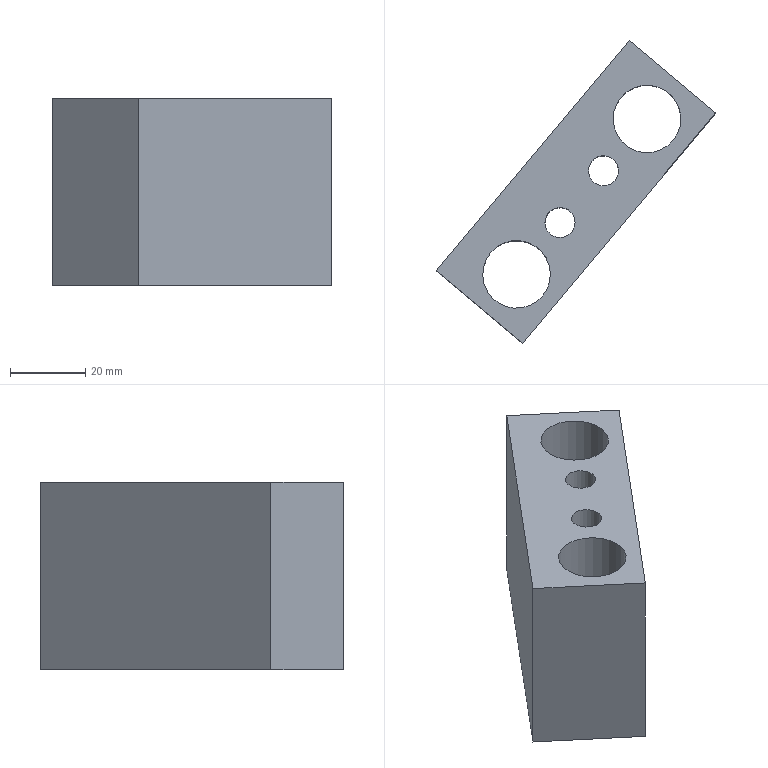Part | NX | features solid 2 | 1 solid | 10 faces | box 74.404 x 80.567 x 50 mm | volume 89527 mm3 | plane 6 | cylinder 4 | commonest cylinder face diameters 8 x2 18 x2
STEP:
#1=CARTESIAN_POINT('',(-632.193,404.46,-40.));
#2=VERTEX_POINT('',#1);
#3=CARTESIAN_POINT('',(-635.257,407.031,-40.));
#4=DIRECTION('',(0.,0.,1.));
#5=DIRECTION('',(0.766,-0.6428,0.));
#6=AXIS2_PLACEMENT_3D('',#3,#4,#5);
#7=CIRCLE('',#6,4.);
#8=EDGE_CURVE('',#2,#2,#7,.T.);
#9=ORIENTED_EDGE('',*,*,#8,.T.);
#10=EDGE_LOOP('',(#9));
#11=FACE_BOUND('',#10,.T.);
#12=CARTESIAN_POINT('',(-620.623,418.249,-40.));
#13=VERTEX_POINT('',#12);
#14=CARTESIAN_POINT('',(-623.687,420.82,-40.));
#15=DIRECTION('',(0.,0.,1.));
#16=DIRECTION('',(0.766,-0.6428,0.));
#17=AXIS2_PLACEMENT_3D('',#14,#15,#16);
#18=CIRCLE('',#17,4.);
#19=EDGE_CURVE('',#13,#13,#18,.T.);
#20=ORIENTED_EDGE('',*,*,#19,.T.);
#21=EDGE_LOOP('',(#20));
#22=FACE_BOUND('',#21,.T.);
#23=CARTESIAN_POINT('',(-605.222,428.824,-40.));
#24=VERTEX_POINT('',#23);
#25=CARTESIAN_POINT('',(-612.117,434.609,-40.));
#26=DIRECTION('',(0.,0.,1.));
#27=DIRECTION('',(0.766,-0.6428,0.));
#28=AXIS2_PLACEMENT_3D('',#25,#26,#27);
#29=CIRCLE('',#28,9.);
#30=EDGE_CURVE('',#24,#24,#29,.T.);
#31=ORIENTED_EDGE('',*,*,#30,.T.);
#32=EDGE_LOOP('',(#31));
#33=FACE_BOUND('',#32,.T.);
#34=CARTESIAN_POINT('',(-639.933,387.457,-40.));
#35=VERTEX_POINT('',#34);
#36=CARTESIAN_POINT('',(-646.827,393.242,-40.));
#37=DIRECTION('',(0.,0.,1.));
#38=DIRECTION('',(0.766,-0.6428,0.));
#39=AXIS2_PLACEMENT_3D('',#36,#37,#38);
#40=CIRCLE('',#39,9.);
#41=EDGE_CURVE('',#35,#35,#40,.T.);
#42=ORIENTED_EDGE('',*,*,#41,.T.);
#43=EDGE_LOOP('',(#42));
#44=FACE_BOUND('',#43,.T.);
#45=CARTESIAN_POINT('',(-616.783,455.495,-40.));
#46=VERTEX_POINT('',#45);
#47=CARTESIAN_POINT('',(-593.802,436.211,-40.));
#48=VERTEX_POINT('',#47);
#49=CARTESIAN_POINT('',(-569.288,415.642,-40.));
#50=DIRECTION('',(0.766,-0.6428,0.));
#51=VECTOR('',#50,1000.);
#52=LINE('',#49,#51);
#53=EDGE_CURVE('',#46,#48,#52,.T.);
#54=ORIENTED_EDGE('',*,*,#53,.T.);
#55=CARTESIAN_POINT('',(-645.225,374.927,-40.));
#56=VERTEX_POINT('',#55);
#57=CARTESIAN_POINT('',(-593.802,436.211,-40.));
#58=DIRECTION('',(-0.6428,-0.766,0.));
#59=VECTOR('',#58,1000.);
#60=LINE('',#57,#59);
#61=EDGE_CURVE('',#48,#56,#60,.T.);
#62=ORIENTED_EDGE('',*,*,#61,.T.);
#63=CARTESIAN_POINT('',(-668.206,394.211,-40.));
#64=VERTEX_POINT('',#63);
#65=CARTESIAN_POINT('',(-620.712,354.358,-40.));
#66=DIRECTION('',(0.766,-0.6428,0.));
#67=VECTOR('',#66,1000.);
#68=LINE('',#65,#67);
#69=EDGE_CURVE('',#64,#56,#68,.T.);
#70=ORIENTED_EDGE('',*,*,#69,.F.);
#71=CARTESIAN_POINT('',(-616.783,455.495,-40.));
#72=DIRECTION('',(-0.6428,-0.766,0.));
#73=VECTOR('',#72,1000.);
#74=LINE('',#71,#73);
#75=EDGE_CURVE('',#46,#64,#74,.T.);
#76=ORIENTED_EDGE('',*,*,#75,.F.);
#77=EDGE_LOOP('',(#54,#62,#70,#76));
#78=FACE_BOUND('',#77,.T.);
#79=CARTESIAN_POINT('',(-569.288,415.642,-40.));
#80=DIRECTION('',(0.,0.,-1.));
#81=DIRECTION('',(-0.6428,-0.766,0.));
#82=AXIS2_PLACEMENT_3D('',#79,#80,#81);
#83=PLANE('',#82);
#84=ADVANCED_FACE('',(#11,#22,#33,#44,#78),#83,.T.);
#85=ORIENTED_EDGE('',*,*,#69,.T.);
#86=CARTESIAN_POINT('',(-645.225,374.927,10.));
#87=VERTEX_POINT('',#86);
#88=CARTESIAN_POINT('',(-645.225,374.927,-40.));
#89=DIRECTION('',(0.,0.,1.));
#90=VECTOR('',#89,1000.);
#91=LINE('',#88,#90);
#92=EDGE_CURVE('',#56,#87,#91,.T.);
#93=ORIENTED_EDGE('',*,*,#92,.T.);
#94=CARTESIAN_POINT('',(-668.206,394.211,10.));
#95=VERTEX_POINT('',#94);
#96=CARTESIAN_POINT('',(-620.712,354.358,10.));
#97=DIRECTION('',(0.766,-0.6428,0.));
#98=VECTOR('',#97,1000.);
#99=LINE('',#96,#98);
#100=EDGE_CURVE('',#95,#87,#99,.T.);
#101=ORIENTED_EDGE('',*,*,#100,.F.);
#102=CARTESIAN_POINT('',(-668.206,394.211,-40.));
#103=DIRECTION('',(0.,0.,1.));
#104=VECTOR('',#103,1000.);
#105=LINE('',#102,#104);
#106=EDGE_CURVE('',#64,#95,#105,.T.);
#107=ORIENTED_EDGE('',*,*,#106,.F.);
#108=EDGE_LOOP('',(#85,#93,#101,#107));
#109=FACE_BOUND('',#108,.T.);
#110=CARTESIAN_POINT('',(-620.712,354.358,-40.));
#111=DIRECTION('',(-0.6428,-0.766,0.));
#112=DIRECTION('',(0.,0.,1.));
#113=AXIS2_PLACEMENT_3D('',#110,#111,#112);
#114=PLANE('',#113);
#115=ADVANCED_FACE('',(#109),#114,.T.);
#116=CARTESIAN_POINT('',(-632.193,404.46,10.));
#117=VERTEX_POINT('',#116);
#118=CARTESIAN_POINT('',(-635.257,407.031,10.));
#119=DIRECTION('',(0.,0.,1.));
#120=DIRECTION('',(0.766,-0.6428,0.));
#121=AXIS2_PLACEMENT_3D('',#118,#119,#120);
#122=CIRCLE('',#121,4.);
#123=EDGE_CURVE('',#117,#117,#122,.T.);
#124=ORIENTED_EDGE('',*,*,#123,.F.);
#125=EDGE_LOOP('',(#124));
#126=FACE_BOUND('',#125,.T.);
#127=CARTESIAN_POINT('',(-620.623,418.249,10.));
#128=VERTEX_POINT('',#127);
#129=CARTESIAN_POINT('',(-623.687,420.82,10.));
#130=DIRECTION('',(0.,0.,1.));
#131=DIRECTION('',(0.766,-0.6428,0.));
#132=AXIS2_PLACEMENT_3D('',#129,#130,#131);
#133=CIRCLE('',#132,4.);
#134=EDGE_CURVE('',#128,#128,#133,.T.);
#135=ORIENTED_EDGE('',*,*,#134,.F.);
#136=EDGE_LOOP('',(#135));
#137=FACE_BOUND('',#136,.T.);
#138=CARTESIAN_POINT('',(-605.222,428.824,10.));
#139=VERTEX_POINT('',#138);
#140=CARTESIAN_POINT('',(-612.117,434.609,10.));
#141=DIRECTION('',(0.,0.,1.));
#142=DIRECTION('',(0.766,-0.6428,0.));
#143=AXIS2_PLACEMENT_3D('',#140,#141,#142);
#144=CIRCLE('',#143,9.);
#145=EDGE_CURVE('',#139,#139,#144,.T.);
#146=ORIENTED_EDGE('',*,*,#145,.F.);
#147=EDGE_LOOP('',(#146));
#148=FACE_BOUND('',#147,.T.);
#149=CARTESIAN_POINT('',(-639.933,387.457,10.));
#150=VERTEX_POINT('',#149);
#151=CARTESIAN_POINT('',(-646.827,393.242,10.));
#152=DIRECTION('',(0.,0.,1.));
#153=DIRECTION('',(0.766,-0.6428,0.));
#154=AXIS2_PLACEMENT_3D('',#151,#152,#153);
#155=CIRCLE('',#154,9.);
#156=EDGE_CURVE('',#150,#150,#155,.T.);
#157=ORIENTED_EDGE('',*,*,#156,.F.);
#158=EDGE_LOOP('',(#157));
#159=FACE_BOUND('',#158,.T.);
#160=ORIENTED_EDGE('',*,*,#100,.T.);
#161=CARTESIAN_POINT('',(-593.802,436.211,10.));
#162=VERTEX_POINT('',#161);
#163=CARTESIAN_POINT('',(-593.802,436.211,10.));
#164=DIRECTION('',(-0.6428,-0.766,0.));
#165=VECTOR('',#164,1000.);
#166=LINE('',#163,#165);
#167=EDGE_CURVE('',#162,#87,#166,.T.);
#168=ORIENTED_EDGE('',*,*,#167,.F.);
#169=CARTESIAN_POINT('',(-616.783,455.495,10.));
#170=VERTEX_POINT('',#169);
#171=CARTESIAN_POINT('',(-569.288,415.642,10.));
#172=DIRECTION('',(0.766,-0.6428,0.));
#173=VECTOR('',#172,1000.);
#174=LINE('',#171,#173);
#175=EDGE_CURVE('',#170,#162,#174,.T.);
#176=ORIENTED_EDGE('',*,*,#175,.F.);
#177=CARTESIAN_POINT('',(-616.783,455.495,10.));
#178=DIRECTION('',(0.6428,0.766,0.));
#179=VECTOR('',#178,1000.);
#180=LINE('',#177,#179);
#181=EDGE_CURVE('',#170,#95,#180,.F.);
#182=ORIENTED_EDGE('',*,*,#181,.T.);
#183=EDGE_LOOP('',(#160,#168,#176,#182));
#184=FACE_BOUND('',#183,.T.);
#185=CARTESIAN_POINT('',(-569.288,415.642,10.));
#186=DIRECTION('',(0.,0.,-1.));
#187=DIRECTION('',(-0.6428,-0.766,0.));
#188=AXIS2_PLACEMENT_3D('',#185,#186,#187);
#189=PLANE('',#188);
#190=ADVANCED_FACE('',(#126,#137,#148,#159,#184),#189,.F.);
#191=CARTESIAN_POINT('',(-616.783,455.495,-40.));
#192=DIRECTION('',(0.,0.,-1.));
#193=VECTOR('',#192,1000.);
#194=LINE('',#191,#193);
#195=EDGE_CURVE('',#46,#170,#194,.F.);
#196=ORIENTED_EDGE('',*,*,#195,.T.);
#197=ORIENTED_EDGE('',*,*,#175,.T.);
#198=CARTESIAN_POINT('',(-593.802,436.211,-40.));
#199=DIRECTION('',(0.,0.,1.));
#200=VECTOR('',#199,1000.);
#201=LINE('',#198,#200);
#202=EDGE_CURVE('',#48,#162,#201,.T.);
#203=ORIENTED_EDGE('',*,*,#202,.F.);
#204=ORIENTED_EDGE('',*,*,#53,.F.);
#205=EDGE_LOOP('',(#196,#197,#203,#204));
#206=FACE_BOUND('',#205,.T.);
#207=CARTESIAN_POINT('',(-569.288,415.642,-40.));
#208=DIRECTION('',(-0.6428,-0.766,0.));
#209=DIRECTION('',(0.,0.,1.));
#210=AXIS2_PLACEMENT_3D('',#207,#208,#209);
#211=PLANE('',#210);
#212=ADVANCED_FACE('',(#206),#211,.F.);
#213=ORIENTED_EDGE('',*,*,#167,.T.);
#214=ORIENTED_EDGE('',*,*,#92,.F.);
#215=ORIENTED_EDGE('',*,*,#61,.F.);
#216=ORIENTED_EDGE('',*,*,#202,.T.);
#217=EDGE_LOOP('',(#213,#214,#215,#216));
#218=FACE_BOUND('',#217,.T.);
#219=CARTESIAN_POINT('',(-593.802,436.211,-40.));
#220=DIRECTION('',(0.766,-0.6428,0.));
#221=DIRECTION('',(-0.6428,-0.766,0.));
#222=AXIS2_PLACEMENT_3D('',#219,#220,#221);
#223=PLANE('',#222);
#224=ADVANCED_FACE('',(#218),#223,.T.);
#225=ORIENTED_EDGE('',*,*,#181,.F.);
#226=ORIENTED_EDGE('',*,*,#195,.F.);
#227=ORIENTED_EDGE('',*,*,#75,.T.);
#228=ORIENTED_EDGE('',*,*,#106,.T.);
#229=EDGE_LOOP('',(#225,#226,#227,#228));
#230=FACE_BOUND('',#229,.T.);
#231=CARTESIAN_POINT('',(-616.783,455.495,-40.));
#232=DIRECTION('',(0.766,-0.6428,0.));
#233=DIRECTION('',(-0.6428,-0.766,0.));
#234=AXIS2_PLACEMENT_3D('',#231,#232,#233);
#235=PLANE('',#234);
#236=ADVANCED_FACE('',(#230),#235,.F.);
#237=ORIENTED_EDGE('',*,*,#41,.F.);
#238=EDGE_LOOP('',(#237));
#239=FACE_BOUND('',#238,.T.);
#240=ORIENTED_EDGE('',*,*,#156,.T.);
#241=EDGE_LOOP('',(#240));
#242=FACE_BOUND('',#241,.T.);
#243=CARTESIAN_POINT('',(-646.827,393.242,10.));
#244=DIRECTION('',(0.,0.,-1.));
#245=DIRECTION('',(0.766,-0.6428,0.));
#246=AXIS2_PLACEMENT_3D('',#243,#244,#245);
#247=CYLINDRICAL_SURFACE('',#246,9.);
#248=ADVANCED_FACE('',(#239,#242),#247,.F.);
#249=ORIENTED_EDGE('',*,*,#30,.F.);
#250=EDGE_LOOP('',(#249));
#251=FACE_BOUND('',#250,.T.);
#252=ORIENTED_EDGE('',*,*,#145,.T.);
#253=EDGE_LOOP('',(#252));
#254=FACE_BOUND('',#253,.T.);
#255=CARTESIAN_POINT('',(-612.117,434.609,10.));
#256=DIRECTION('',(0.,0.,-1.));
#257=DIRECTION('',(0.766,-0.6428,0.));
#258=AXIS2_PLACEMENT_3D('',#255,#256,#257);
#259=CYLINDRICAL_SURFACE('',#258,9.);
#260=ADVANCED_FACE('',(#251,#254),#259,.F.);
#261=ORIENTED_EDGE('',*,*,#19,.F.);
#262=EDGE_LOOP('',(#261));
#263=FACE_BOUND('',#262,.T.);
#264=ORIENTED_EDGE('',*,*,#134,.T.);
#265=EDGE_LOOP('',(#264));
#266=FACE_BOUND('',#265,.T.);
#267=CARTESIAN_POINT('',(-623.687,420.82,10.));
#268=DIRECTION('',(0.,0.,-1.));
#269=DIRECTION('',(0.766,-0.6428,0.));
#270=AXIS2_PLACEMENT_3D('',#267,#268,#269);
#271=CYLINDRICAL_SURFACE('',#270,4.);
#272=ADVANCED_FACE('',(#263,#266),#271,.F.);
#273=ORIENTED_EDGE('',*,*,#8,.F.);
#274=EDGE_LOOP('',(#273));
#275=FACE_BOUND('',#274,.T.);
#276=ORIENTED_EDGE('',*,*,#123,.T.);
#277=EDGE_LOOP('',(#276));
#278=FACE_BOUND('',#277,.T.);
#279=CARTESIAN_POINT('',(-635.257,407.031,10.));
#280=DIRECTION('',(0.,0.,-1.));
#281=DIRECTION('',(0.766,-0.6428,0.));
#282=AXIS2_PLACEMENT_3D('',#279,#280,#281);
#283=CYLINDRICAL_SURFACE('',#282,4.);
#284=ADVANCED_FACE('',(#275,#278),#283,.F.);
#285=CLOSED_SHELL('',(#84,#115,#190,#212,#224,#236,#248,#260,#272,#284));
#286=MANIFOLD_SOLID_BREP('',#285);
#287=(LENGTH_UNIT()NAMED_UNIT(*)SI_UNIT(.MILLI.,.METRE.));
#288=UNCERTAINTY_MEASURE_WITH_UNIT(LENGTH_MEASURE(0.00001),#287,'','');
#289=(NAMED_UNIT(*)PLANE_ANGLE_UNIT()SI_UNIT($,.RADIAN.));
#290=(NAMED_UNIT(*)SI_UNIT($,.STERADIAN.)SOLID_ANGLE_UNIT());
#291=(GEOMETRIC_REPRESENTATION_CONTEXT(3)GLOBAL_UNCERTAINTY_ASSIGNED_CONTEXT((#288))GLOBAL_UNIT_ASSIGNED_CONTEXT((#287,#289,#290))REPRESENTATION_CONTEXT('',''));
#292=ADVANCED_BREP_SHAPE_REPRESENTATION('',(#286),#291);